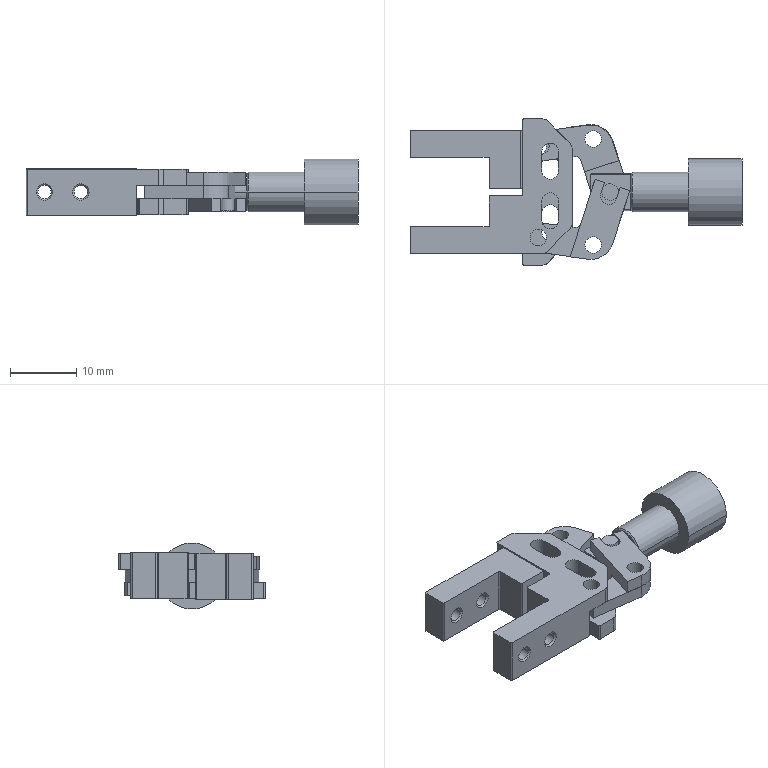Part | SolidWorks | features BaseBody 1 | 1 solid | 182 faces | box 50.2 x 22.1 x 10 mm | volume 3109 mm3 | plane 91 | cylinder 71 | cone 20 | commonest cylinder face diameters 2.5 x22 0.4 x12 2 x10 2.013 x8 2.52 x6 7 x4